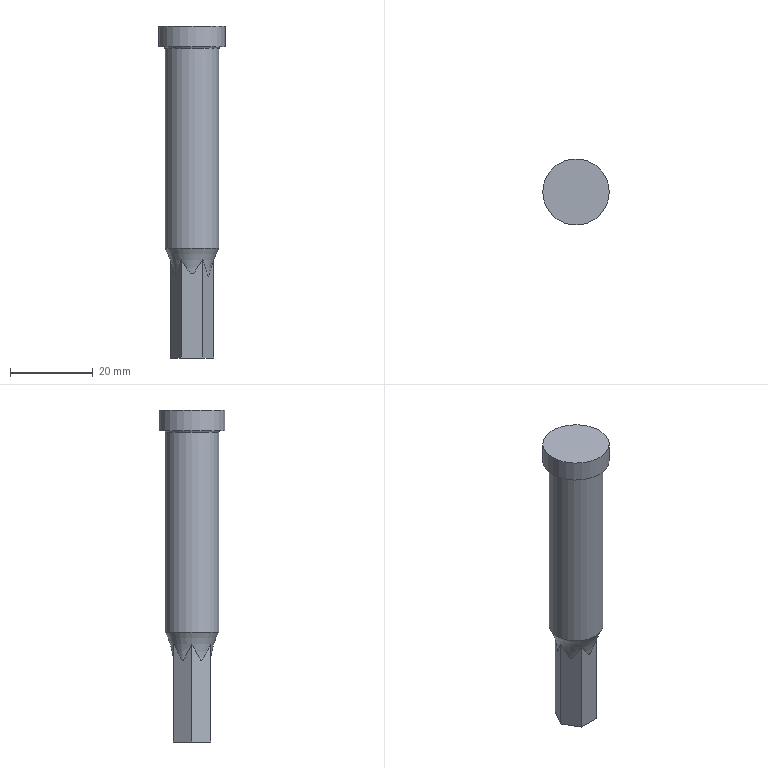Part | NX | features solid 2 | 1 solid | 13 faces | box 16 x 16 x 80 mm | volume 9445 mm3 | plane 5 | spline 4 | cylinder 2 | torus 2 | commonest cylinder face diameters 13 x1 16 x1
STEP:
#1=CARTESIAN_POINT('',(105.512,-352.381,8.));
#2=VERTEX_POINT('',#1);
#3=CARTESIAN_POINT('',(112.512,-352.381,8.));
#4=DIRECTION('',(0.,0.,-1.));
#5=DIRECTION('',(-1.,0.,0.));
#6=AXIS2_PLACEMENT_3D('',#3,#4,#5);
#7=CIRCLE('',#6,7.);
#8=EDGE_CURVE('',#2,#2,#7,.F.);
#9=ORIENTED_EDGE('',*,*,#8,.T.);
#10=EDGE_LOOP('',(#9));
#11=FACE_BOUND('',#10,.T.);
#12=CARTESIAN_POINT('',(104.512,-352.381,8.));
#13=VERTEX_POINT('',#12);
#14=CARTESIAN_POINT('',(112.512,-352.381,8.));
#15=DIRECTION('',(0.,0.,-1.));
#16=DIRECTION('',(-1.,0.,0.));
#17=AXIS2_PLACEMENT_3D('',#14,#15,#16);
#18=CIRCLE('',#17,8.);
#19=EDGE_CURVE('',#13,#13,#18,.T.);
#20=ORIENTED_EDGE('',*,*,#19,.T.);
#21=EDGE_LOOP('',(#20));
#22=FACE_BOUND('',#21,.T.);
#23=CARTESIAN_POINT('',(112.512,-352.381,8.));
#24=DIRECTION('',(0.,0.,-1.));
#25=DIRECTION('',(-1.,0.,0.));
#26=AXIS2_PLACEMENT_3D('',#23,#24,#25);
#27=PLANE('',#26);
#28=ADVANCED_FACE('',(#11,#22),#27,.T.);
#29=ORIENTED_EDGE('',*,*,#19,.F.);
#30=EDGE_LOOP('',(#29));
#31=FACE_BOUND('',#30,.T.);
#32=CARTESIAN_POINT('',(120.512,-352.381,13.));
#33=VERTEX_POINT('',#32);
#34=CARTESIAN_POINT('',(112.512,-352.381,13.));
#35=DIRECTION('',(0.,0.,1.));
#36=DIRECTION('',(1.,0.,0.));
#37=AXIS2_PLACEMENT_3D('',#34,#35,#36);
#38=CIRCLE('',#37,8.);
#39=EDGE_CURVE('',#33,#33,#38,.F.);
#40=ORIENTED_EDGE('',*,*,#39,.T.);
#41=EDGE_LOOP('',(#40));
#42=FACE_BOUND('',#41,.T.);
#43=CARTESIAN_POINT('',(112.512,-352.381,8.));
#44=DIRECTION('',(0.,0.,1.));
#45=DIRECTION('',(1.,0.,0.));
#46=AXIS2_PLACEMENT_3D('',#43,#44,#45);
#47=CYLINDRICAL_SURFACE('',#46,8.);
#48=ADVANCED_FACE('',(#31,#42),#47,.T.);
#49=ORIENTED_EDGE('',*,*,#39,.F.);
#50=EDGE_LOOP('',(#49));
#51=FACE_BOUND('',#50,.T.);
#52=CARTESIAN_POINT('',(112.512,-352.381,13.));
#53=DIRECTION('',(0.,0.,-1.));
#54=DIRECTION('',(-1.,0.,0.));
#55=AXIS2_PLACEMENT_3D('',#52,#53,#54);
#56=PLANE('',#55);
#57=ADVANCED_FACE('',(#51),#56,.F.);
#58=CARTESIAN_POINT('',(106.012,-352.381,7.5));
#59=VERTEX_POINT('',#58);
#60=CARTESIAN_POINT('',(112.512,-352.381,7.5));
#61=DIRECTION('',(0.,0.,-1.));
#62=DIRECTION('',(-1.,0.,0.));
#63=AXIS2_PLACEMENT_3D('',#60,#61,#62);
#64=CIRCLE('',#63,6.5);
#65=EDGE_CURVE('',#59,#59,#64,.T.);
#66=ORIENTED_EDGE('',*,*,#65,.T.);
#67=EDGE_LOOP('',(#66));
#68=FACE_BOUND('',#67,.T.);
#69=CARTESIAN_POINT('',(106.012,-352.381,-40.517));
#70=VERTEX_POINT('',#69);
#71=CARTESIAN_POINT('',(112.512,-352.381,-40.517));
#72=DIRECTION('',(0.,0.,-1.));
#73=DIRECTION('',(-1.,0.,0.));
#74=AXIS2_PLACEMENT_3D('',#71,#72,#73);
#75=CIRCLE('',#74,6.5);
#76=EDGE_CURVE('',#70,#70,#75,.T.);
#77=ORIENTED_EDGE('',*,*,#76,.F.);
#78=EDGE_LOOP('',(#77));
#79=FACE_BOUND('',#78,.T.);
#80=CARTESIAN_POINT('',(112.512,-352.381,-42.276));
#81=DIRECTION('',(0.,0.,1.));
#82=DIRECTION('',(1.,0.,0.));
#83=AXIS2_PLACEMENT_3D('',#80,#81,#82);
#84=CYLINDRICAL_SURFACE('',#83,6.5);
#85=ADVANCED_FACE('',(#68,#79),#84,.T.);
#86=ORIENTED_EDGE('',*,*,#65,.F.);
#87=EDGE_LOOP('',(#86));
#88=FACE_BOUND('',#87,.T.);
#89=ORIENTED_EDGE('',*,*,#8,.F.);
#90=EDGE_LOOP('',(#89));
#91=FACE_BOUND('',#90,.T.);
#92=CARTESIAN_POINT('',(112.512,-352.381,7.5));
#93=DIRECTION('',(0.,0.,-1.));
#94=DIRECTION('',(-1.,0.,0.));
#95=AXIS2_PLACEMENT_3D('',#92,#93,#94);
#96=TOROIDAL_SURFACE('',#95,7.,0.5);
#97=ADVANCED_FACE('',(#88,#91),#96,.F.);
#98=ORIENTED_EDGE('',*,*,#76,.T.);
#99=EDGE_LOOP('',(#98));
#100=FACE_BOUND('',#99,.T.);
#101=CARTESIAN_POINT('',(115.11,-356.935,-43.336));
#102=VERTEX_POINT('',#101);
#103=CARTESIAN_POINT('',(109.914,-356.935,-43.336));
#104=VERTEX_POINT('',#103);
#105=CARTESIAN_POINT('',(115.11,-356.935,-43.336));
#106=CARTESIAN_POINT('',(114.421,-356.935,-44.379));
#107=CARTESIAN_POINT('',(113.43,-356.928,-46.025));
#108=CARTESIAN_POINT('',(112.61,-356.938,-46.997));
#109=CARTESIAN_POINT('',(111.723,-356.933,-46.254));
#110=CARTESIAN_POINT('',(110.67,-356.935,-44.481));
#111=CARTESIAN_POINT('',(109.914,-356.935,-43.336));
#112=B_SPLINE_CURVE_WITH_KNOTS('',3,(#105,#106,#107,#108,#109,#110,#111),.UNSPECIFIED.,.F.,.F.,(4,1,1,1,4),(0.,0.25,0.5,0.75,1.),.UNSPECIFIED.);
#113=EDGE_CURVE('',#102,#104,#112,.T.);
#114=ORIENTED_EDGE('',*,*,#113,.F.);
#115=CARTESIAN_POINT('',(117.708,-352.381,-43.483));
#116=VERTEX_POINT('',#115);
#117=CARTESIAN_POINT('',(117.708,-352.381,-43.483));
#118=CARTESIAN_POINT('',(117.604,-352.563,-43.812));
#119=CARTESIAN_POINT('',(117.45,-352.834,-44.317));
#120=CARTESIAN_POINT('',(117.279,-353.134,-44.891));
#121=CARTESIAN_POINT('',(117.172,-353.321,-45.253));
#122=CARTESIAN_POINT('',(117.119,-353.414,-45.434));
#123=CARTESIAN_POINT('',(116.964,-353.686,-45.962));
#124=CARTESIAN_POINT('',(116.82,-353.94,-46.446));
#125=CARTESIAN_POINT('',(116.591,-354.346,-47.153));
#126=CARTESIAN_POINT('',(116.422,-354.632,-47.519));
#127=CARTESIAN_POINT('',(116.26,-354.925,-47.107));
#128=CARTESIAN_POINT('',(116.025,-355.332,-46.378));
#129=CARTESIAN_POINT('',(115.878,-355.59,-45.882));
#130=CARTESIAN_POINT('',(115.722,-355.864,-45.348));
#131=CARTESIAN_POINT('',(115.665,-355.962,-45.157));
#132=CARTESIAN_POINT('',(115.555,-356.155,-44.784));
#133=CARTESIAN_POINT('',(115.378,-356.466,-44.192));
#134=CARTESIAN_POINT('',(115.218,-356.747,-43.673));
#135=CARTESIAN_POINT('',(115.11,-356.935,-43.336));
#136=B_SPLINE_CURVE_WITH_KNOTS('',3,(#117,#118,#119,#120,#121,#122,#123,#124,#125,#126,#127,#128,#129,#130,#131,#132,#133,#134,#135),.UNSPECIFIED.,.F.,.F.,(4,1,1,1,1,1,1,1,1,1,1,1,1,1,1,1,4),(0.,0.125,0.1875,0.2188,0.25,0.2812,0.3125,0.375,0.5,0.625,0.6875,0.7188,0.75,0.7812,0.8125,0.875,1.),.UNSPECIFIED.);
#137=EDGE_CURVE('',#116,#102,#136,.T.);
#138=ORIENTED_EDGE('',*,*,#137,.F.);
#139=CARTESIAN_POINT('',(115.11,-347.826,-43.336));
#140=VERTEX_POINT('',#139);
#141=CARTESIAN_POINT('',(115.11,-347.826,-43.336));
#142=CARTESIAN_POINT('',(115.216,-348.012,-43.669));
#143=CARTESIAN_POINT('',(115.424,-348.375,-44.34));
#144=CARTESIAN_POINT('',(115.675,-348.816,-45.188));
#145=CARTESIAN_POINT('',(115.874,-349.165,-45.87));
#146=CARTESIAN_POINT('',(116.025,-349.429,-46.378));
#147=CARTESIAN_POINT('',(116.153,-349.654,-46.806));
#148=CARTESIAN_POINT('',(116.265,-349.851,-47.116));
#149=CARTESIAN_POINT('',(116.365,-350.026,-47.383));
#150=CARTESIAN_POINT('',(116.526,-350.309,-47.331));
#151=CARTESIAN_POINT('',(116.646,-350.519,-46.989));
#152=CARTESIAN_POINT('',(116.837,-350.853,-46.414));
#153=CARTESIAN_POINT('',(117.086,-351.29,-45.538));
#154=CARTESIAN_POINT('',(117.392,-351.826,-44.506));
#155=CARTESIAN_POINT('',(117.601,-352.193,-43.822));
#156=CARTESIAN_POINT('',(117.708,-352.381,-43.483));
#157=B_SPLINE_CURVE_WITH_KNOTS('',3,(#141,#142,#143,#144,#145,#146,#147,#148,#149,#150,#151,#152,#153,#154,#155,#156),.UNSPECIFIED.,.F.,.F.,(4,1,1,1,1,1,1,1,1,1,1,1,1,4),(0.,0.001186,0.002373,0.002966,0.003559,0.004152,0.004449,0.004746,0.005042,0.005339,0.005932,0.007118,0.008305,0.009491),.UNSPECIFIED.);
#158=EDGE_CURVE('',#140,#116,#157,.T.);
#159=ORIENTED_EDGE('',*,*,#158,.F.);
#160=CARTESIAN_POINT('',(109.914,-347.826,-43.336));
#161=VERTEX_POINT('',#160);
#162=CARTESIAN_POINT('',(109.914,-347.826,-43.336));
#163=CARTESIAN_POINT('',(110.603,-347.826,-44.38));
#164=CARTESIAN_POINT('',(111.595,-347.833,-46.025));
#165=CARTESIAN_POINT('',(112.415,-347.824,-46.997));
#166=CARTESIAN_POINT('',(113.302,-347.828,-46.254));
#167=CARTESIAN_POINT('',(114.354,-347.826,-44.481));
#168=CARTESIAN_POINT('',(115.11,-347.826,-43.336));
#169=B_SPLINE_CURVE_WITH_KNOTS('',3,(#162,#163,#164,#165,#166,#167,#168),.UNSPECIFIED.,.F.,.F.,(4,1,1,1,4),(0.,0.25,0.5,0.75,1.),.UNSPECIFIED.);
#170=EDGE_CURVE('',#161,#140,#169,.T.);
#171=ORIENTED_EDGE('',*,*,#170,.F.);
#172=CARTESIAN_POINT('',(107.316,-352.381,-43.483));
#173=VERTEX_POINT('',#172);
#174=CARTESIAN_POINT('',(107.316,-352.381,-43.483));
#175=CARTESIAN_POINT('',(107.42,-352.199,-43.812));
#176=CARTESIAN_POINT('',(107.575,-351.927,-44.317));
#177=CARTESIAN_POINT('',(107.746,-351.628,-44.891));
#178=CARTESIAN_POINT('',(107.852,-351.44,-45.253));
#179=CARTESIAN_POINT('',(107.906,-351.347,-45.434));
#180=CARTESIAN_POINT('',(108.06,-351.076,-45.962));
#181=CARTESIAN_POINT('',(108.204,-350.821,-46.446));
#182=CARTESIAN_POINT('',(108.433,-350.416,-47.153));
#183=CARTESIAN_POINT('',(108.602,-350.129,-47.519));
#184=CARTESIAN_POINT('',(108.765,-349.836,-47.107));
#185=CARTESIAN_POINT('',(108.999,-349.429,-46.378));
#186=CARTESIAN_POINT('',(109.146,-349.172,-45.882));
#187=CARTESIAN_POINT('',(109.303,-348.898,-45.348));
#188=CARTESIAN_POINT('',(109.359,-348.799,-45.157));
#189=CARTESIAN_POINT('',(109.469,-348.606,-44.784));
#190=CARTESIAN_POINT('',(109.647,-348.295,-44.192));
#191=CARTESIAN_POINT('',(109.807,-348.014,-43.673));
#192=CARTESIAN_POINT('',(109.914,-347.826,-43.336));
#193=B_SPLINE_CURVE_WITH_KNOTS('',3,(#174,#175,#176,#177,#178,#179,#180,#181,#182,#183,#184,#185,#186,#187,#188,#189,#190,#191,#192),.UNSPECIFIED.,.F.,.F.,(4,1,1,1,1,1,1,1,1,1,1,1,1,1,1,1,4),(0.,0.125,0.1875,0.2188,0.25,0.2812,0.3125,0.375,0.5,0.625,0.6875,0.7188,0.75,0.7812,0.8125,0.875,1.),.UNSPECIFIED.);
#194=EDGE_CURVE('',#173,#161,#193,.T.);
#195=ORIENTED_EDGE('',*,*,#194,.F.);
#196=CARTESIAN_POINT('',(109.914,-356.935,-43.336));
#197=CARTESIAN_POINT('',(109.808,-356.75,-43.669));
#198=CARTESIAN_POINT('',(109.601,-356.386,-44.34));
#199=CARTESIAN_POINT('',(109.349,-355.945,-45.188));
#200=CARTESIAN_POINT('',(109.15,-355.596,-45.87));
#201=CARTESIAN_POINT('',(109.,-355.333,-46.378));
#202=CARTESIAN_POINT('',(108.872,-355.108,-46.806));
#203=CARTESIAN_POINT('',(108.759,-354.91,-47.116));
#204=CARTESIAN_POINT('',(108.659,-354.736,-47.383));
#205=CARTESIAN_POINT('',(108.498,-354.453,-47.331));
#206=CARTESIAN_POINT('',(108.378,-354.243,-46.989));
#207=CARTESIAN_POINT('',(108.187,-353.908,-46.414));
#208=CARTESIAN_POINT('',(107.938,-353.471,-45.538));
#209=CARTESIAN_POINT('',(107.632,-352.935,-44.506));
#210=CARTESIAN_POINT('',(107.423,-352.568,-43.822));
#211=CARTESIAN_POINT('',(107.316,-352.381,-43.483));
#212=B_SPLINE_CURVE_WITH_KNOTS('',3,(#196,#197,#198,#199,#200,#201,#202,#203,#204,#205,#206,#207,#208,#209,#210,#211),.UNSPECIFIED.,.F.,.F.,(4,1,1,1,1,1,1,1,1,1,1,1,1,4),(0.,0.001186,0.002373,0.002966,0.003559,0.004152,0.004449,0.004746,0.005042,0.005339,0.005932,0.007118,0.008305,0.009491),.UNSPECIFIED.);
#213=EDGE_CURVE('',#104,#173,#212,.T.);
#214=ORIENTED_EDGE('',*,*,#213,.F.);
#215=EDGE_LOOP('',(#114,#138,#159,#171,#195,#214));
#216=FACE_BOUND('',#215,.T.);
#217=CARTESIAN_POINT('',(112.512,-352.381,-48.));
#218=DIRECTION('',(0.,0.,1.));
#219=DIRECTION('',(-1.,0.,0.));
#220=AXIS2_PLACEMENT_3D('',#217,#218,#219);
#221=TOROIDAL_SURFACE('',#220,19.5,15.);
#222=ADVANCED_FACE('',(#100,#216),#221,.F.);
#223=CARTESIAN_POINT('',(115.11,-356.935,-67.));
#224=VERTEX_POINT('',#223);
#225=CARTESIAN_POINT('',(109.914,-356.935,-67.));
#226=VERTEX_POINT('',#225);
#227=CARTESIAN_POINT('',(115.11,-356.935,-67.));
#228=CARTESIAN_POINT('',(113.378,-356.935,-67.));
#229=CARTESIAN_POINT('',(111.646,-356.935,-67.));
#230=CARTESIAN_POINT('',(109.914,-356.935,-67.));
#231=B_SPLINE_CURVE_WITH_KNOTS('',3,(#227,#228,#229,#230),.UNSPECIFIED.,.F.,.F.,(4,4),(0.,0.005196),.UNSPECIFIED.);
#232=EDGE_CURVE('',#224,#226,#231,.T.);
#233=ORIENTED_EDGE('',*,*,#232,.T.);
#234=CARTESIAN_POINT('',(107.316,-352.381,-67.));
#235=VERTEX_POINT('',#234);
#236=CARTESIAN_POINT('',(107.316,-352.381,-67.));
#237=DIRECTION('',(-0.4955,0.8686,0.));
#238=VECTOR('',#237,1000.);
#239=LINE('',#236,#238);
#240=EDGE_CURVE('',#226,#235,#239,.T.);
#241=ORIENTED_EDGE('',*,*,#240,.T.);
#242=CARTESIAN_POINT('',(109.914,-347.826,-67.));
#243=VERTEX_POINT('',#242);
#244=CARTESIAN_POINT('',(107.316,-352.381,-67.));
#245=CARTESIAN_POINT('',(108.182,-350.862,-67.));
#246=CARTESIAN_POINT('',(109.048,-349.344,-67.));
#247=CARTESIAN_POINT('',(109.914,-347.826,-67.));
#248=B_SPLINE_CURVE_WITH_KNOTS('',3,(#244,#245,#246,#247),.UNSPECIFIED.,.F.,.F.,(4,4),(0.,0.005244),.UNSPECIFIED.);
#249=EDGE_CURVE('',#235,#243,#248,.T.);
#250=ORIENTED_EDGE('',*,*,#249,.T.);
#251=CARTESIAN_POINT('',(115.11,-347.826,-67.));
#252=VERTEX_POINT('',#251);
#253=CARTESIAN_POINT('',(109.914,-347.826,-67.));
#254=CARTESIAN_POINT('',(111.646,-347.826,-67.));
#255=CARTESIAN_POINT('',(113.378,-347.826,-67.));
#256=CARTESIAN_POINT('',(115.11,-347.826,-67.));
#257=B_SPLINE_CURVE_WITH_KNOTS('',3,(#253,#254,#255,#256),.UNSPECIFIED.,.F.,.F.,(4,4),(0.,0.005196),.UNSPECIFIED.);
#258=EDGE_CURVE('',#243,#252,#257,.T.);
#259=ORIENTED_EDGE('',*,*,#258,.T.);
#260=CARTESIAN_POINT('',(117.708,-352.381,-67.));
#261=VERTEX_POINT('',#260);
#262=CARTESIAN_POINT('',(117.708,-352.381,-67.));
#263=DIRECTION('',(0.4955,-0.8686,0.));
#264=VECTOR('',#263,1000.);
#265=LINE('',#262,#264);
#266=EDGE_CURVE('',#252,#261,#265,.T.);
#267=ORIENTED_EDGE('',*,*,#266,.T.);
#268=CARTESIAN_POINT('',(117.708,-352.381,-67.));
#269=CARTESIAN_POINT('',(116.842,-353.899,-67.));
#270=CARTESIAN_POINT('',(115.976,-355.417,-67.));
#271=CARTESIAN_POINT('',(115.11,-356.935,-67.));
#272=B_SPLINE_CURVE_WITH_KNOTS('',3,(#268,#269,#270,#271),.UNSPECIFIED.,.F.,.F.,(4,4),(0.,0.005244),.UNSPECIFIED.);
#273=EDGE_CURVE('',#261,#224,#272,.T.);
#274=ORIENTED_EDGE('',*,*,#273,.T.);
#275=EDGE_LOOP('',(#233,#241,#250,#259,#267,#274));
#276=FACE_BOUND('',#275,.T.);
#277=CARTESIAN_POINT('',(0.,0.,-67.));
#278=DIRECTION('',(0.,0.,1.));
#279=DIRECTION('',(-1.,0.,0.));
#280=AXIS2_PLACEMENT_3D('',#277,#278,#279);
#281=PLANE('',#280);
#282=ADVANCED_FACE('',(#276),#281,.F.);
#283=ORIENTED_EDGE('',*,*,#194,.T.);
#284=CARTESIAN_POINT('',(109.914,-347.826,-53.291));
#285=DIRECTION('',(0.,0.,1.));
#286=VECTOR('',#285,1000.);
#287=LINE('',#284,#286);
#288=EDGE_CURVE('',#161,#243,#287,.F.);
#289=ORIENTED_EDGE('',*,*,#288,.T.);
#290=ORIENTED_EDGE('',*,*,#249,.F.);
#291=CARTESIAN_POINT('',(107.316,-352.381,-53.339));
#292=DIRECTION('',(0.,0.,1.));
#293=VECTOR('',#292,1000.);
#294=LINE('',#291,#293);
#295=EDGE_CURVE('',#235,#173,#294,.T.);
#296=ORIENTED_EDGE('',*,*,#295,.T.);
#297=EDGE_LOOP('',(#283,#289,#290,#296));
#298=FACE_BOUND('',#297,.T.);
#299=CARTESIAN_POINT('',(109.914,-347.826,-67.334));
#300=CARTESIAN_POINT('',(109.914,-347.826,-43.193));
#301=CARTESIAN_POINT('',(109.052,-349.338,-67.271));
#302=CARTESIAN_POINT('',(109.052,-349.338,-43.129));
#303=CARTESIAN_POINT('',(108.186,-350.856,-67.207));
#304=CARTESIAN_POINT('',(108.186,-350.856,-43.066));
#305=CARTESIAN_POINT('',(107.316,-352.381,-67.143));
#306=CARTESIAN_POINT('',(107.316,-352.381,-43.002));
#307=B_SPLINE_SURFACE_WITH_KNOTS('',3,1,((#299,#300),(#301,#302),(#303,#304),(#305,#306)),.SURF_OF_LINEAR_EXTRUSION.,.F.,.F.,.F.,(4,4),(2,2),(0.8328,1.),(0.,1.),.PIECEWISE_BEZIER_KNOTS.);
#308=ADVANCED_FACE('',(#298),#307,.T.);
#309=ORIENTED_EDGE('',*,*,#170,.T.);
#310=CARTESIAN_POINT('',(115.11,-347.826,-53.291));
#311=DIRECTION('',(0.,0.,1.));
#312=VECTOR('',#311,1000.);
#313=LINE('',#310,#312);
#314=EDGE_CURVE('',#140,#252,#313,.F.);
#315=ORIENTED_EDGE('',*,*,#314,.T.);
#316=ORIENTED_EDGE('',*,*,#258,.F.);
#317=ORIENTED_EDGE('',*,*,#288,.F.);
#318=EDGE_LOOP('',(#309,#315,#316,#317));
#319=FACE_BOUND('',#318,.T.);
#320=CARTESIAN_POINT('',(115.11,-347.826,-67.));
#321=CARTESIAN_POINT('',(115.11,-347.826,-43.194));
#322=CARTESIAN_POINT('',(113.378,-347.826,-67.));
#323=CARTESIAN_POINT('',(113.378,-347.826,-43.194));
#324=CARTESIAN_POINT('',(111.646,-347.826,-67.));
#325=CARTESIAN_POINT('',(111.646,-347.826,-43.194));
#326=CARTESIAN_POINT('',(109.914,-347.826,-67.));
#327=CARTESIAN_POINT('',(109.914,-347.826,-43.194));
#328=B_SPLINE_SURFACE_WITH_KNOTS('',3,1,((#320,#321),(#322,#323),(#324,#325),(#326,#327)),.SURF_OF_LINEAR_EXTRUSION.,.F.,.F.,.F.,(4,4),(2,2),(0.6672,0.8328),(0.,1.),.PIECEWISE_BEZIER_KNOTS.);
#329=ADVANCED_FACE('',(#319),#328,.T.);
#330=ORIENTED_EDGE('',*,*,#158,.T.);
#331=CARTESIAN_POINT('',(117.708,-352.381,-53.337));
#332=DIRECTION('',(0.,0.,1.));
#333=VECTOR('',#332,1000.);
#334=LINE('',#331,#333);
#335=EDGE_CURVE('',#116,#261,#334,.F.);
#336=ORIENTED_EDGE('',*,*,#335,.T.);
#337=ORIENTED_EDGE('',*,*,#266,.F.);
#338=ORIENTED_EDGE('',*,*,#314,.F.);
#339=EDGE_LOOP('',(#330,#336,#337,#338));
#340=FACE_BOUND('',#339,.T.);
#341=CARTESIAN_POINT('',(117.708,-352.381,-64.));
#342=DIRECTION('',(-0.8686,-0.4955,0.));
#343=DIRECTION('',(-0.4955,0.8686,0.));
#344=AXIS2_PLACEMENT_3D('',#341,#342,#343);
#345=PLANE('',#344);
#346=ADVANCED_FACE('',(#340),#345,.F.);
#347=ORIENTED_EDGE('',*,*,#137,.T.);
#348=CARTESIAN_POINT('',(115.11,-356.935,-53.339));
#349=DIRECTION('',(0.,0.,1.));
#350=VECTOR('',#349,1000.);
#351=LINE('',#348,#350);
#352=EDGE_CURVE('',#224,#102,#351,.T.);
#353=ORIENTED_EDGE('',*,*,#352,.F.);
#354=ORIENTED_EDGE('',*,*,#273,.F.);
#355=ORIENTED_EDGE('',*,*,#335,.F.);
#356=EDGE_LOOP('',(#347,#353,#354,#355));
#357=FACE_BOUND('',#356,.T.);
#358=CARTESIAN_POINT('',(115.11,-356.935,-67.142));
#359=CARTESIAN_POINT('',(115.11,-356.935,-43.15));
#360=CARTESIAN_POINT('',(115.98,-355.411,-67.206));
#361=CARTESIAN_POINT('',(115.98,-355.411,-43.214));
#362=CARTESIAN_POINT('',(116.846,-353.893,-67.27));
#363=CARTESIAN_POINT('',(116.846,-353.893,-43.278));
#364=CARTESIAN_POINT('',(117.708,-352.381,-67.334));
#365=CARTESIAN_POINT('',(117.708,-352.381,-43.341));
#366=B_SPLINE_SURFACE_WITH_KNOTS('',3,1,((#358,#359),(#360,#361),(#362,#363),(#364,#365)),.SURF_OF_LINEAR_EXTRUSION.,.F.,.F.,.F.,(4,4),(2,2),(0.3328,0.5),(0.,1.),.PIECEWISE_BEZIER_KNOTS.);
#367=ADVANCED_FACE('',(#357),#366,.T.);
#368=ORIENTED_EDGE('',*,*,#113,.T.);
#369=CARTESIAN_POINT('',(109.914,-356.935,-53.339));
#370=DIRECTION('',(0.,0.,1.));
#371=VECTOR('',#370,1000.);
#372=LINE('',#369,#371);
#373=EDGE_CURVE('',#226,#104,#372,.T.);
#374=ORIENTED_EDGE('',*,*,#373,.F.);
#375=ORIENTED_EDGE('',*,*,#232,.F.);
#376=ORIENTED_EDGE('',*,*,#352,.T.);
#377=EDGE_LOOP('',(#368,#374,#375,#376));
#378=FACE_BOUND('',#377,.T.);
#379=CARTESIAN_POINT('',(109.914,-356.935,-67.));
#380=CARTESIAN_POINT('',(109.914,-356.935,-43.194));
#381=CARTESIAN_POINT('',(111.646,-356.935,-67.));
#382=CARTESIAN_POINT('',(111.646,-356.935,-43.194));
#383=CARTESIAN_POINT('',(113.378,-356.935,-67.));
#384=CARTESIAN_POINT('',(113.378,-356.935,-43.194));
#385=CARTESIAN_POINT('',(115.11,-356.935,-67.));
#386=CARTESIAN_POINT('',(115.11,-356.935,-43.194));
#387=B_SPLINE_SURFACE_WITH_KNOTS('',3,1,((#379,#380),(#381,#382),(#383,#384),(#385,#386)),.SURF_OF_LINEAR_EXTRUSION.,.F.,.F.,.F.,(4,4),(2,2),(0.1672,0.3328),(0.,1.),.PIECEWISE_BEZIER_KNOTS.);
#388=ADVANCED_FACE('',(#378),#387,.T.);
#389=ORIENTED_EDGE('',*,*,#213,.T.);
#390=ORIENTED_EDGE('',*,*,#295,.F.);
#391=ORIENTED_EDGE('',*,*,#240,.F.);
#392=ORIENTED_EDGE('',*,*,#373,.T.);
#393=EDGE_LOOP('',(#389,#390,#391,#392));
#394=FACE_BOUND('',#393,.T.);
#395=CARTESIAN_POINT('',(107.316,-352.381,-64.));
#396=DIRECTION('',(0.8686,0.4955,0.));
#397=DIRECTION('',(0.4955,-0.8686,0.));
#398=AXIS2_PLACEMENT_3D('',#395,#396,#397);
#399=PLANE('',#398);
#400=ADVANCED_FACE('',(#394),#399,.F.);
#401=CLOSED_SHELL('',(#28,#48,#57,#85,#97,#222,#282,#308,#329,#346,#367,#388,#400));
#402=MANIFOLD_SOLID_BREP('',#401);
#403=(LENGTH_UNIT()NAMED_UNIT(*)SI_UNIT(.MILLI.,.METRE.));
#404=UNCERTAINTY_MEASURE_WITH_UNIT(LENGTH_MEASURE(0.0508),#403,'','');
#405=(NAMED_UNIT(*)PLANE_ANGLE_UNIT()SI_UNIT($,.RADIAN.));
#406=(NAMED_UNIT(*)SI_UNIT($,.STERADIAN.)SOLID_ANGLE_UNIT());
#407=(GEOMETRIC_REPRESENTATION_CONTEXT(3)GLOBAL_UNCERTAINTY_ASSIGNED_CONTEXT((#404))GLOBAL_UNIT_ASSIGNED_CONTEXT((#403,#405,#406))REPRESENTATION_CONTEXT('',''));
#408=ADVANCED_BREP_SHAPE_REPRESENTATION('',(#402),#407);